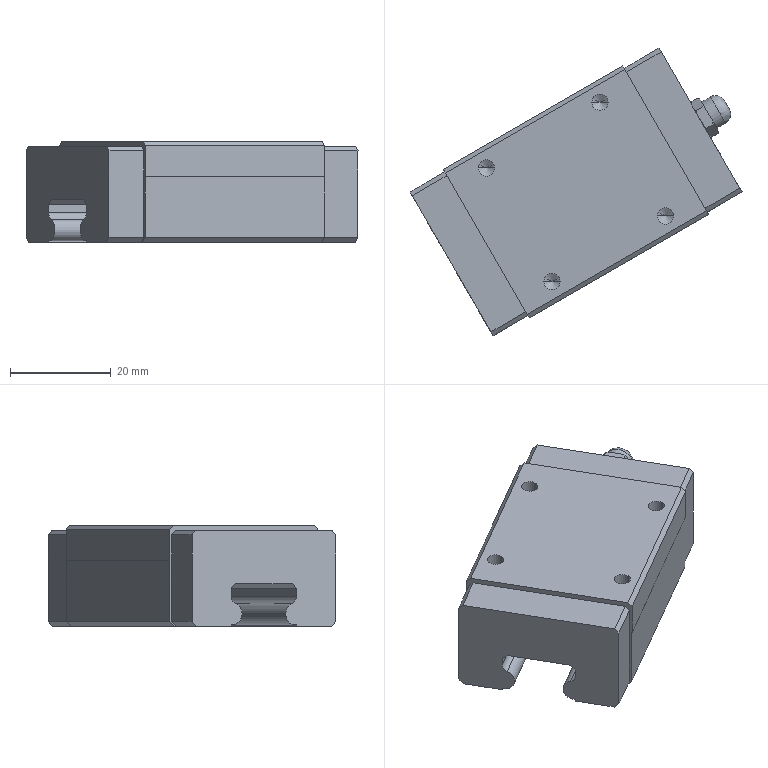Part | SolidWorks | features BaseBody 1 | 1 solid | 85 faces | box 65.813 x 56.992 x 20 mm | volume 31433 mm3 | plane 46 | cone 22 | cylinder 15 | spline 2 | commonest cylinder face diameters 3.242 x8 4.4 x3 3 x2 6 x2